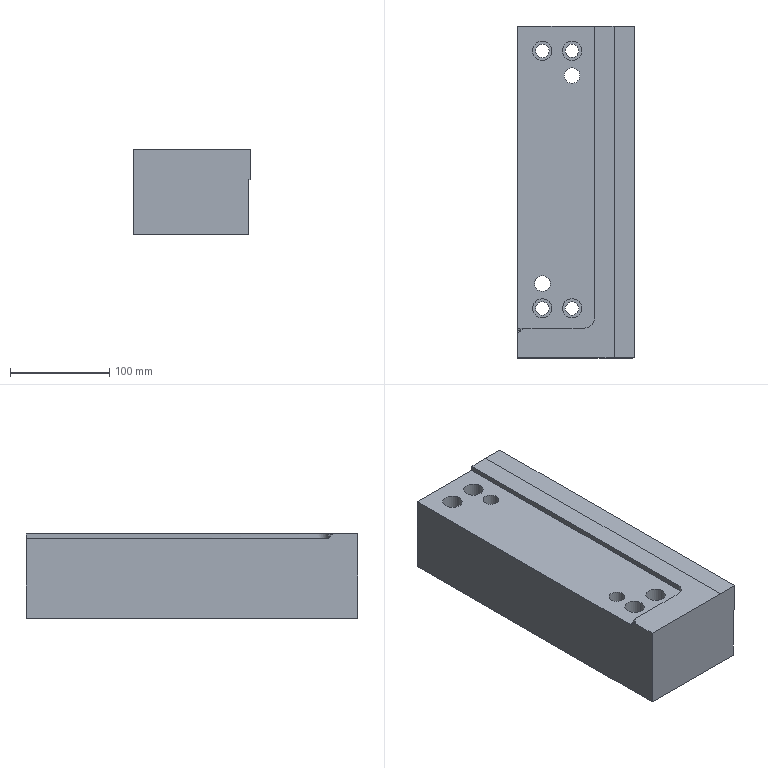Part | NX | features solid 2 | 1 solid | 31 faces | box 117.712 x 335 x 85 mm | volume 3079659 mm3 | spline 12 | cylinder 10 | plane 9 | commonest cylinder face diameters 13.5 x4 19.5 x4 16 x2